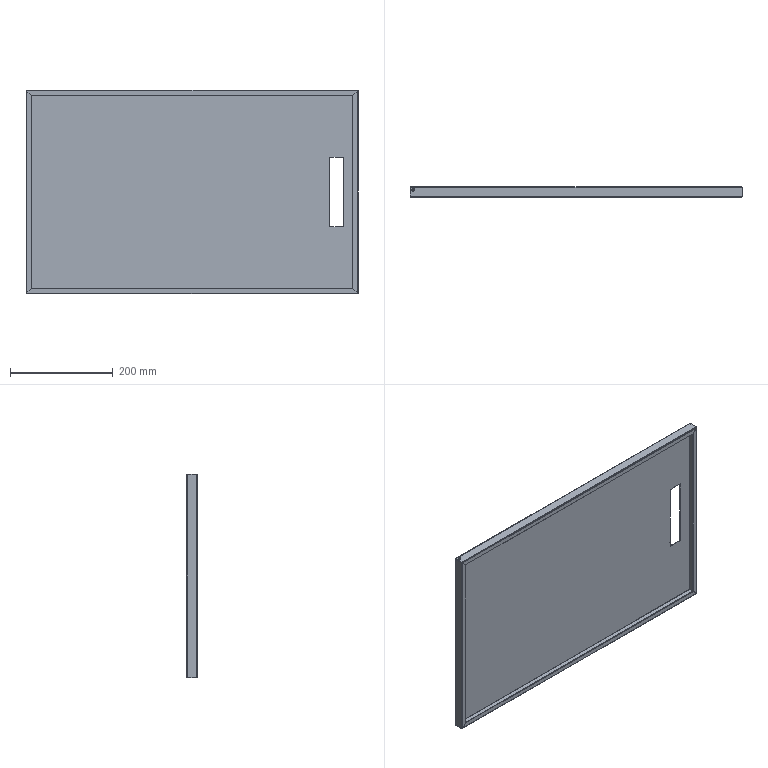Part | SolidWorks | features BaseBody 1 | 1 solid | 94 faces | box 645 x 20 x 396 mm | volume 458573 mm3 | plane 66 | cylinder 20 | spline 8 | commonest cylinder face diameters 0.4 x8 3.4 x8 5.1 x4